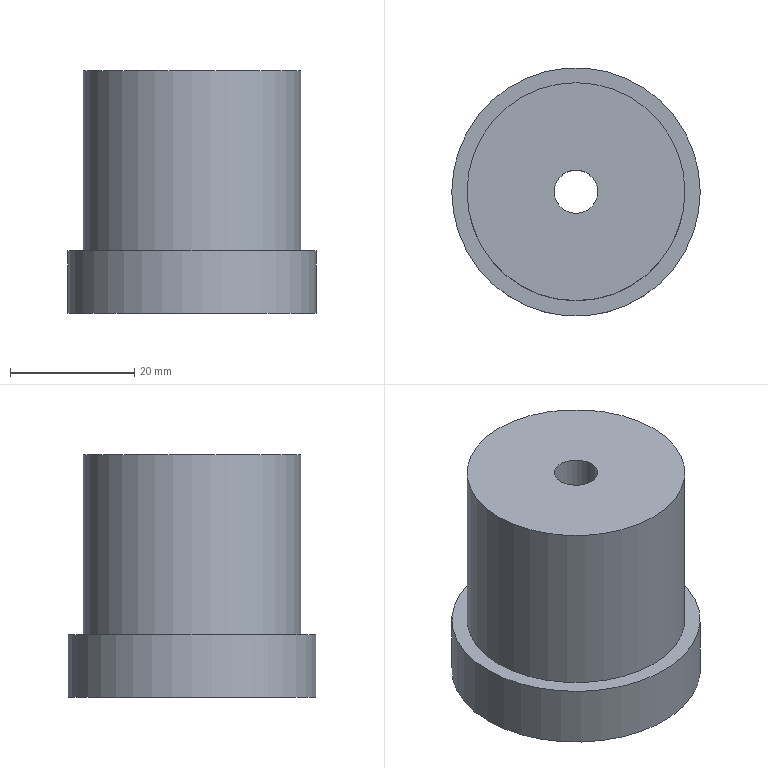Part | NX | features solid 2 | 1 solid | 8 faces | box 40 x 40 x 39 mm | volume 32293 mm3 | plane 4 | cylinder 4 | commonest cylinder face diameters 7 x1 22 x1 35.1 x1 40 x1
STEP:
#1=CARTESIAN_POINT('',(1537.616,80.895,15.));
#2=VERTEX_POINT('',#1);
#3=CARTESIAN_POINT('',(1534.116,80.895,15.));
#4=DIRECTION('',(0.,0.,1.));
#5=DIRECTION('',(1.,0.,0.));
#6=AXIS2_PLACEMENT_3D('',#3,#4,#5);
#7=CIRCLE('',#6,3.5);
#8=EDGE_CURVE('',#2,#2,#7,.T.);
#9=ORIENTED_EDGE('',*,*,#8,.F.);
#10=EDGE_LOOP('',(#9));
#11=FACE_BOUND('',#10,.T.);
#12=CARTESIAN_POINT('',(1516.566,80.895,15.));
#13=VERTEX_POINT('',#12);
#14=CARTESIAN_POINT('',(1534.116,80.895,15.));
#15=DIRECTION('',(0.,0.,-1.));
#16=DIRECTION('',(-1.,0.,0.));
#17=AXIS2_PLACEMENT_3D('',#14,#15,#16);
#18=CIRCLE('',#17,17.55);
#19=EDGE_CURVE('',#13,#13,#18,.F.);
#20=ORIENTED_EDGE('',*,*,#19,.T.);
#21=EDGE_LOOP('',(#20));
#22=FACE_BOUND('',#21,.T.);
#23=CARTESIAN_POINT('',(1543.188,80.753,15.));
#24=DIRECTION('',(0.,0.,1.));
#25=DIRECTION('',(-1.,0.,0.));
#26=AXIS2_PLACEMENT_3D('',#23,#24,#25);
#27=PLANE('',#26);
#28=ADVANCED_FACE('',(#11,#22),#27,.T.);
#29=CARTESIAN_POINT('',(1516.566,80.895,-14.));
#30=VERTEX_POINT('',#29);
#31=CARTESIAN_POINT('',(1534.116,80.895,-14.));
#32=DIRECTION('',(0.,0.,-1.));
#33=DIRECTION('',(-1.,0.,0.));
#34=AXIS2_PLACEMENT_3D('',#31,#32,#33);
#35=CIRCLE('',#34,17.55);
#36=EDGE_CURVE('',#30,#30,#35,.F.);
#37=ORIENTED_EDGE('',*,*,#36,.T.);
#38=EDGE_LOOP('',(#37));
#39=FACE_BOUND('',#38,.T.);
#40=ORIENTED_EDGE('',*,*,#19,.F.);
#41=EDGE_LOOP('',(#40));
#42=FACE_BOUND('',#41,.T.);
#43=CARTESIAN_POINT('',(1534.116,80.895,6.));
#44=DIRECTION('',(0.,0.,-1.));
#45=DIRECTION('',(1.,0.,0.));
#46=AXIS2_PLACEMENT_3D('',#43,#44,#45);
#47=CYLINDRICAL_SURFACE('',#46,17.55);
#48=ADVANCED_FACE('',(#39,#42),#47,.T.);
#49=CARTESIAN_POINT('',(1514.116,80.895,-24.));
#50=VERTEX_POINT('',#49);
#51=CARTESIAN_POINT('',(1534.116,80.895,-24.));
#52=DIRECTION('',(0.,0.,-1.));
#53=DIRECTION('',(-1.,0.,0.));
#54=AXIS2_PLACEMENT_3D('',#51,#52,#53);
#55=CIRCLE('',#54,20.);
#56=EDGE_CURVE('',#50,#50,#55,.F.);
#57=ORIENTED_EDGE('',*,*,#56,.F.);
#58=EDGE_LOOP('',(#57));
#59=FACE_BOUND('',#58,.T.);
#60=CARTESIAN_POINT('',(1523.116,80.895,-24.));
#61=VERTEX_POINT('',#60);
#62=CARTESIAN_POINT('',(1534.116,80.895,-24.));
#63=DIRECTION('',(0.,0.,-1.));
#64=DIRECTION('',(-1.,0.,0.));
#65=AXIS2_PLACEMENT_3D('',#62,#63,#64);
#66=CIRCLE('',#65,11.);
#67=EDGE_CURVE('',#61,#61,#66,.F.);
#68=ORIENTED_EDGE('',*,*,#67,.T.);
#69=EDGE_LOOP('',(#68));
#70=FACE_BOUND('',#69,.T.);
#71=CARTESIAN_POINT('',(1534.116,80.895,-24.));
#72=DIRECTION('',(0.,0.,1.));
#73=DIRECTION('',(-1.,0.,0.));
#74=AXIS2_PLACEMENT_3D('',#71,#72,#73);
#75=PLANE('',#74);
#76=ADVANCED_FACE('',(#59,#70),#75,.F.);
#77=ORIENTED_EDGE('',*,*,#36,.F.);
#78=EDGE_LOOP('',(#77));
#79=FACE_BOUND('',#78,.T.);
#80=CARTESIAN_POINT('',(1514.116,80.895,-14.));
#81=VERTEX_POINT('',#80);
#82=CARTESIAN_POINT('',(1534.116,80.895,-14.));
#83=DIRECTION('',(0.,0.,-1.));
#84=DIRECTION('',(-1.,0.,0.));
#85=AXIS2_PLACEMENT_3D('',#82,#83,#84);
#86=CIRCLE('',#85,20.);
#87=EDGE_CURVE('',#81,#81,#86,.F.);
#88=ORIENTED_EDGE('',*,*,#87,.T.);
#89=EDGE_LOOP('',(#88));
#90=FACE_BOUND('',#89,.T.);
#91=CARTESIAN_POINT('',(1534.116,80.895,-14.));
#92=DIRECTION('',(0.,0.,1.));
#93=DIRECTION('',(-1.,0.,0.));
#94=AXIS2_PLACEMENT_3D('',#91,#92,#93);
#95=PLANE('',#94);
#96=ADVANCED_FACE('',(#79,#90),#95,.T.);
#97=ORIENTED_EDGE('',*,*,#56,.T.);
#98=EDGE_LOOP('',(#97));
#99=FACE_BOUND('',#98,.T.);
#100=ORIENTED_EDGE('',*,*,#87,.F.);
#101=EDGE_LOOP('',(#100));
#102=FACE_BOUND('',#101,.T.);
#103=CARTESIAN_POINT('',(1534.116,80.895,-14.));
#104=DIRECTION('',(0.,0.,-1.));
#105=DIRECTION('',(1.,0.,0.));
#106=AXIS2_PLACEMENT_3D('',#103,#104,#105);
#107=CYLINDRICAL_SURFACE('',#106,20.);
#108=ADVANCED_FACE('',(#99,#102),#107,.T.);
#109=CARTESIAN_POINT('',(1537.616,80.895,-4.));
#110=VERTEX_POINT('',#109);
#111=CARTESIAN_POINT('',(1534.116,80.895,-4.));
#112=DIRECTION('',(0.,0.,1.));
#113=DIRECTION('',(1.,0.,0.));
#114=AXIS2_PLACEMENT_3D('',#111,#112,#113);
#115=CIRCLE('',#114,3.5);
#116=EDGE_CURVE('',#110,#110,#115,.T.);
#117=ORIENTED_EDGE('',*,*,#116,.T.);
#118=EDGE_LOOP('',(#117));
#119=FACE_BOUND('',#118,.T.);
#120=CARTESIAN_POINT('',(1523.116,80.895,-4.));
#121=VERTEX_POINT('',#120);
#122=CARTESIAN_POINT('',(1534.116,80.895,-4.));
#123=DIRECTION('',(0.,0.,-1.));
#124=DIRECTION('',(-1.,0.,0.));
#125=AXIS2_PLACEMENT_3D('',#122,#123,#124);
#126=CIRCLE('',#125,11.);
#127=EDGE_CURVE('',#121,#121,#126,.T.);
#128=ORIENTED_EDGE('',*,*,#127,.T.);
#129=EDGE_LOOP('',(#128));
#130=FACE_BOUND('',#129,.T.);
#131=CARTESIAN_POINT('',(1534.116,80.895,-4.));
#132=DIRECTION('',(0.,0.,1.));
#133=DIRECTION('',(-1.,0.,0.));
#134=AXIS2_PLACEMENT_3D('',#131,#132,#133);
#135=PLANE('',#134);
#136=ADVANCED_FACE('',(#119,#130),#135,.F.);
#137=ORIENTED_EDGE('',*,*,#127,.F.);
#138=EDGE_LOOP('',(#137));
#139=FACE_BOUND('',#138,.T.);
#140=ORIENTED_EDGE('',*,*,#67,.F.);
#141=EDGE_LOOP('',(#140));
#142=FACE_BOUND('',#141,.T.);
#143=CARTESIAN_POINT('',(1534.116,80.895,-14.));
#144=DIRECTION('',(0.,0.,1.));
#145=DIRECTION('',(-1.,0.,0.));
#146=AXIS2_PLACEMENT_3D('',#143,#144,#145);
#147=CYLINDRICAL_SURFACE('',#146,11.);
#148=ADVANCED_FACE('',(#139,#142),#147,.F.);
#149=ORIENTED_EDGE('',*,*,#8,.T.);
#150=EDGE_LOOP('',(#149));
#151=FACE_BOUND('',#150,.T.);
#152=ORIENTED_EDGE('',*,*,#116,.F.);
#153=EDGE_LOOP('',(#152));
#154=FACE_BOUND('',#153,.T.);
#155=CARTESIAN_POINT('',(1534.116,80.895,-204.));
#156=DIRECTION('',(0.,0.,1.));
#157=DIRECTION('',(1.,0.,0.));
#158=AXIS2_PLACEMENT_3D('',#155,#156,#157);
#159=CYLINDRICAL_SURFACE('',#158,3.5);
#160=ADVANCED_FACE('',(#151,#154),#159,.F.);
#161=CLOSED_SHELL('',(#28,#48,#76,#96,#108,#136,#148,#160));
#162=MANIFOLD_SOLID_BREP('',#161);
#163=(LENGTH_UNIT()NAMED_UNIT(*)SI_UNIT(.MILLI.,.METRE.));
#164=UNCERTAINTY_MEASURE_WITH_UNIT(LENGTH_MEASURE(0.00001),#163,'','');
#165=(NAMED_UNIT(*)PLANE_ANGLE_UNIT()SI_UNIT($,.RADIAN.));
#166=(NAMED_UNIT(*)SI_UNIT($,.STERADIAN.)SOLID_ANGLE_UNIT());
#167=(GEOMETRIC_REPRESENTATION_CONTEXT(3)GLOBAL_UNCERTAINTY_ASSIGNED_CONTEXT((#164))GLOBAL_UNIT_ASSIGNED_CONTEXT((#163,#165,#166))REPRESENTATION_CONTEXT('',''));
#168=ADVANCED_BREP_SHAPE_REPRESENTATION('',(#162),#167);